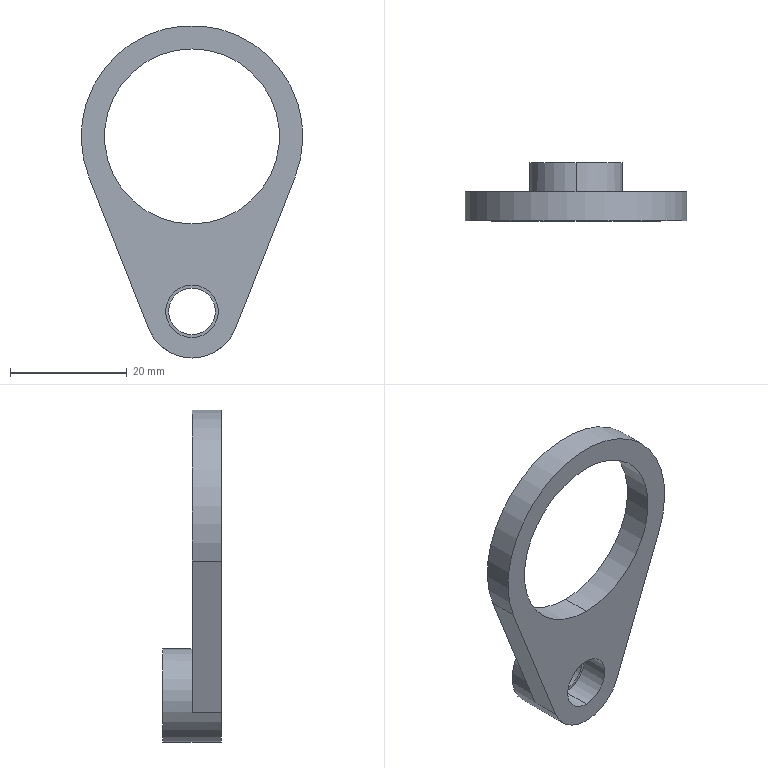Part | SolidWorks | features ICE 3, Extrusion 1 | 1 solid | 15 faces | box 38 x 10 x 57 mm | volume 4565 mm3 | cylinder 9 | plane 6 | commonest cylinder face diameters 8 x2 9 x2 16 x2 30 x2 38 x1
STEP:
#1=CARTESIAN_POINT('',(0.,5.,4.5));
#2=VERTEX_POINT('',#1);
#3=CARTESIAN_POINT('',(0.,5.,-4.5));
#4=VERTEX_POINT('',#3);
#5=CARTESIAN_POINT('',(0.,5.,0.));
#6=DIRECTION('',(0.,-1.,0.));
#7=DIRECTION('',(0.,0.,-1.));
#8=AXIS2_PLACEMENT_3D('',#5,#6,#7);
#9=CIRCLE('',#8,4.5);
#10=EDGE_CURVE('',#2,#4,#9,.T.);
#11=ORIENTED_EDGE('',*,*,#10,.F.);
#12=CARTESIAN_POINT('',(0.,0.,4.5));
#13=VERTEX_POINT('',#12);
#14=CARTESIAN_POINT('',(0.,5.,4.5));
#15=DIRECTION('',(0.,-1.,0.));
#16=VECTOR('',#15,1000.);
#17=LINE('',#14,#16);
#18=EDGE_CURVE('',#2,#13,#17,.T.);
#19=ORIENTED_EDGE('',*,*,#18,.T.);
#20=CARTESIAN_POINT('',(0.,0.,-4.5));
#21=VERTEX_POINT('',#20);
#22=CARTESIAN_POINT('',(0.,0.,0.));
#23=DIRECTION('',(0.,-1.,0.));
#24=DIRECTION('',(0.,0.,-1.));
#25=AXIS2_PLACEMENT_3D('',#22,#23,#24);
#26=CIRCLE('',#25,4.5);
#27=EDGE_CURVE('',#13,#21,#26,.T.);
#28=ORIENTED_EDGE('',*,*,#27,.T.);
#29=CARTESIAN_POINT('',(0.,5.,-4.5));
#30=DIRECTION('',(0.,-1.,0.));
#31=VECTOR('',#30,1000.);
#32=LINE('',#29,#31);
#33=EDGE_CURVE('',#4,#21,#32,.T.);
#34=ORIENTED_EDGE('',*,*,#33,.F.);
#35=EDGE_LOOP('',(#11,#19,#28,#34));
#36=FACE_OUTER_BOUND('',#35,.T.);
#37=CARTESIAN_POINT('',(0.,5.,0.));
#38=DIRECTION('',(0.,-1.,0.));
#39=DIRECTION('',(0.,0.,-1.));
#40=AXIS2_PLACEMENT_3D('',#37,#38,#39);
#41=CYLINDRICAL_SURFACE('',#40,4.5);
#42=ADVANCED_FACE('',(#36),#41,.F.);
#43=CARTESIAN_POINT('',(0.,0.,15.));
#44=VERTEX_POINT('',#43);
#45=CARTESIAN_POINT('',(0.,0.,45.));
#46=VERTEX_POINT('',#45);
#47=CARTESIAN_POINT('',(0.,0.,30.));
#48=DIRECTION('',(0.,1.,0.));
#49=DIRECTION('',(0.,0.,1.));
#50=AXIS2_PLACEMENT_3D('',#47,#48,#49);
#51=CIRCLE('',#50,15.);
#52=EDGE_CURVE('',#44,#46,#51,.T.);
#53=ORIENTED_EDGE('',*,*,#52,.F.);
#54=CARTESIAN_POINT('',(0.,5.,15.));
#55=VERTEX_POINT('',#54);
#56=CARTESIAN_POINT('',(0.,-29.,15.));
#57=DIRECTION('',(0.,1.,0.));
#58=VECTOR('',#57,1000.);
#59=LINE('',#56,#58);
#60=EDGE_CURVE('',#44,#55,#59,.T.);
#61=ORIENTED_EDGE('',*,*,#60,.T.);
#62=CARTESIAN_POINT('',(0.,5.,45.));
#63=VERTEX_POINT('',#62);
#64=CARTESIAN_POINT('',(0.,5.,30.));
#65=DIRECTION('',(0.,1.,0.));
#66=DIRECTION('',(0.,0.,1.));
#67=AXIS2_PLACEMENT_3D('',#64,#65,#66);
#68=CIRCLE('',#67,15.);
#69=EDGE_CURVE('',#55,#63,#68,.T.);
#70=ORIENTED_EDGE('',*,*,#69,.T.);
#71=CARTESIAN_POINT('',(0.,-29.,45.));
#72=DIRECTION('',(0.,1.,0.));
#73=VECTOR('',#72,1000.);
#74=LINE('',#71,#73);
#75=EDGE_CURVE('',#46,#63,#74,.T.);
#76=ORIENTED_EDGE('',*,*,#75,.F.);
#77=EDGE_LOOP('',(#53,#61,#70,#76));
#78=FACE_OUTER_BOUND('',#77,.T.);
#79=CARTESIAN_POINT('',(0.,-29.,30.));
#80=DIRECTION('',(0.,1.,0.));
#81=DIRECTION('',(0.,0.,1.));
#82=AXIS2_PLACEMENT_3D('',#79,#80,#81);
#83=CYLINDRICAL_SURFACE('',#82,15.);
#84=ADVANCED_FACE('',(#78),#83,.F.);
#85=CARTESIAN_POINT('',(0.,10.,8.));
#86=VERTEX_POINT('',#85);
#87=CARTESIAN_POINT('',(0.,10.,-8.));
#88=VERTEX_POINT('',#87);
#89=CARTESIAN_POINT('',(0.,10.,0.));
#90=DIRECTION('',(0.,1.,0.));
#91=DIRECTION('',(0.,0.,1.));
#92=AXIS2_PLACEMENT_3D('',#89,#90,#91);
#93=CIRCLE('',#92,8.);
#94=EDGE_CURVE('',#86,#88,#93,.T.);
#95=ORIENTED_EDGE('',*,*,#94,.F.);
#96=CARTESIAN_POINT('',(0.,5.,8.));
#97=VERTEX_POINT('',#96);
#98=CARTESIAN_POINT('',(0.,5.,8.));
#99=DIRECTION('',(0.,-1.,0.));
#100=VECTOR('',#99,1000.);
#101=LINE('',#98,#100);
#102=EDGE_CURVE('',#86,#97,#101,.T.);
#103=ORIENTED_EDGE('',*,*,#102,.T.);
#104=CARTESIAN_POINT('',(7.443,5.,-2.933));
#105=VERTEX_POINT('',#104);
#106=CARTESIAN_POINT('',(0.,5.,0.));
#107=DIRECTION('',(0.,1.,0.));
#108=DIRECTION('',(0.,0.,1.));
#109=AXIS2_PLACEMENT_3D('',#106,#107,#108);
#110=CIRCLE('',#109,8.);
#111=EDGE_CURVE('',#97,#105,#110,.T.);
#112=ORIENTED_EDGE('',*,*,#111,.T.);
#113=CARTESIAN_POINT('',(7.443,0.,-2.933));
#114=VERTEX_POINT('',#113);
#115=CARTESIAN_POINT('',(7.443,5.,-2.933));
#116=DIRECTION('',(0.,-1.,0.));
#117=VECTOR('',#116,1000.);
#118=LINE('',#115,#117);
#119=EDGE_CURVE('',#105,#114,#118,.T.);
#120=ORIENTED_EDGE('',*,*,#119,.T.);
#121=CARTESIAN_POINT('',(0.,0.,-8.));
#122=VERTEX_POINT('',#121);
#123=CARTESIAN_POINT('',(0.,0.,0.));
#124=DIRECTION('',(0.,1.,0.));
#125=DIRECTION('',(0.,0.,1.));
#126=AXIS2_PLACEMENT_3D('',#123,#124,#125);
#127=CIRCLE('',#126,8.);
#128=EDGE_CURVE('',#114,#122,#127,.T.);
#129=ORIENTED_EDGE('',*,*,#128,.T.);
#130=CARTESIAN_POINT('',(0.,5.,-8.));
#131=DIRECTION('',(0.,-1.,0.));
#132=VECTOR('',#131,1000.);
#133=LINE('',#130,#132);
#134=EDGE_CURVE('',#88,#122,#133,.T.);
#135=ORIENTED_EDGE('',*,*,#134,.F.);
#136=EDGE_LOOP('',(#95,#103,#112,#120,#129,#135));
#137=FACE_OUTER_BOUND('',#136,.T.);
#138=CARTESIAN_POINT('',(0.,5.,0.));
#139=DIRECTION('',(0.,-1.,0.));
#140=DIRECTION('',(0.,0.,-1.));
#141=AXIS2_PLACEMENT_3D('',#138,#139,#140);
#142=CYLINDRICAL_SURFACE('',#141,8.);
#143=ADVANCED_FACE('',(#137),#142,.T.);
#144=CARTESIAN_POINT('',(0.,5.,-4.));
#145=VERTEX_POINT('',#144);
#146=CARTESIAN_POINT('',(0.,5.,4.));
#147=VERTEX_POINT('',#146);
#148=CARTESIAN_POINT('',(0.,5.,0.));
#149=DIRECTION('',(0.,1.,0.));
#150=DIRECTION('',(0.,0.,-1.));
#151=AXIS2_PLACEMENT_3D('',#148,#149,#150);
#152=CIRCLE('',#151,4.);
#153=EDGE_CURVE('',#145,#147,#152,.T.);
#154=ORIENTED_EDGE('',*,*,#153,.F.);
#155=CARTESIAN_POINT('',(0.,10.,-4.));
#156=VERTEX_POINT('',#155);
#157=CARTESIAN_POINT('',(0.,-29.,-4.));
#158=DIRECTION('',(0.,1.,0.));
#159=VECTOR('',#158,1000.);
#160=LINE('',#157,#159);
#161=EDGE_CURVE('',#145,#156,#160,.T.);
#162=ORIENTED_EDGE('',*,*,#161,.T.);
#163=CARTESIAN_POINT('',(0.,10.,4.));
#164=VERTEX_POINT('',#163);
#165=CARTESIAN_POINT('',(0.,10.,0.));
#166=DIRECTION('',(0.,1.,0.));
#167=DIRECTION('',(0.,0.,1.));
#168=AXIS2_PLACEMENT_3D('',#165,#166,#167);
#169=CIRCLE('',#168,4.);
#170=EDGE_CURVE('',#156,#164,#169,.T.);
#171=ORIENTED_EDGE('',*,*,#170,.T.);
#172=CARTESIAN_POINT('',(0.,-29.,4.));
#173=DIRECTION('',(0.,1.,0.));
#174=VECTOR('',#173,1000.);
#175=LINE('',#172,#174);
#176=EDGE_CURVE('',#147,#164,#175,.T.);
#177=ORIENTED_EDGE('',*,*,#176,.F.);
#178=EDGE_LOOP('',(#154,#162,#171,#177));
#179=FACE_OUTER_BOUND('',#178,.T.);
#180=CARTESIAN_POINT('',(0.,-29.,0.));
#181=DIRECTION('',(0.,1.,0.));
#182=DIRECTION('',(0.,0.,1.));
#183=AXIS2_PLACEMENT_3D('',#180,#181,#182);
#184=CYLINDRICAL_SURFACE('',#183,4.);
#185=ADVANCED_FACE('',(#179),#184,.F.);
#186=ORIENTED_EDGE('',*,*,#161,.F.);
#187=CARTESIAN_POINT('',(0.,5.,0.));
#188=DIRECTION('',(0.,1.,0.));
#189=DIRECTION('',(0.,0.,-1.));
#190=AXIS2_PLACEMENT_3D('',#187,#188,#189);
#191=CIRCLE('',#190,4.);
#192=EDGE_CURVE('',#147,#145,#191,.T.);
#193=ORIENTED_EDGE('',*,*,#192,.F.);
#194=ORIENTED_EDGE('',*,*,#176,.T.);
#195=CARTESIAN_POINT('',(0.,10.,0.));
#196=DIRECTION('',(0.,1.,0.));
#197=DIRECTION('',(0.,0.,1.));
#198=AXIS2_PLACEMENT_3D('',#195,#196,#197);
#199=CIRCLE('',#198,4.);
#200=EDGE_CURVE('',#164,#156,#199,.T.);
#201=ORIENTED_EDGE('',*,*,#200,.T.);
#202=EDGE_LOOP('',(#186,#193,#194,#201));
#203=FACE_OUTER_BOUND('',#202,.T.);
#204=CARTESIAN_POINT('',(0.,-29.,0.));
#205=DIRECTION('',(0.,1.,0.));
#206=DIRECTION('',(0.,0.,1.));
#207=AXIS2_PLACEMENT_3D('',#204,#205,#206);
#208=CYLINDRICAL_SURFACE('',#207,4.);
#209=ADVANCED_FACE('',(#203),#208,.F.);
#210=ORIENTED_EDGE('',*,*,#102,.F.);
#211=CARTESIAN_POINT('',(0.,10.,0.));
#212=DIRECTION('',(0.,1.,0.));
#213=DIRECTION('',(0.,0.,1.));
#214=AXIS2_PLACEMENT_3D('',#211,#212,#213);
#215=CIRCLE('',#214,8.);
#216=EDGE_CURVE('',#88,#86,#215,.T.);
#217=ORIENTED_EDGE('',*,*,#216,.F.);
#218=ORIENTED_EDGE('',*,*,#134,.T.);
#219=CARTESIAN_POINT('',(-7.443,0.,-2.933));
#220=VERTEX_POINT('',#219);
#221=CARTESIAN_POINT('',(0.,0.,0.));
#222=DIRECTION('',(0.,1.,0.));
#223=DIRECTION('',(0.,0.,1.));
#224=AXIS2_PLACEMENT_3D('',#221,#222,#223);
#225=CIRCLE('',#224,8.);
#226=EDGE_CURVE('',#122,#220,#225,.T.);
#227=ORIENTED_EDGE('',*,*,#226,.T.);
#228=CARTESIAN_POINT('',(-7.443,5.,-2.933));
#229=VERTEX_POINT('',#228);
#230=CARTESIAN_POINT('',(-7.443,5.,-2.933));
#231=DIRECTION('',(0.,-1.,0.));
#232=VECTOR('',#231,1000.);
#233=LINE('',#230,#232);
#234=EDGE_CURVE('',#229,#220,#233,.T.);
#235=ORIENTED_EDGE('',*,*,#234,.F.);
#236=CARTESIAN_POINT('',(0.,5.,0.));
#237=DIRECTION('',(0.,1.,0.));
#238=DIRECTION('',(0.,0.,1.));
#239=AXIS2_PLACEMENT_3D('',#236,#237,#238);
#240=CIRCLE('',#239,8.);
#241=EDGE_CURVE('',#229,#97,#240,.T.);
#242=ORIENTED_EDGE('',*,*,#241,.T.);
#243=EDGE_LOOP('',(#210,#217,#218,#227,#235,#242));
#244=FACE_OUTER_BOUND('',#243,.T.);
#245=CARTESIAN_POINT('',(0.,5.,0.));
#246=DIRECTION('',(0.,-1.,0.));
#247=DIRECTION('',(0.,0.,-1.));
#248=AXIS2_PLACEMENT_3D('',#245,#246,#247);
#249=CYLINDRICAL_SURFACE('',#248,8.);
#250=ADVANCED_FACE('',(#244),#249,.T.);
#251=CARTESIAN_POINT('',(-17.677,0.,23.033));
#252=VERTEX_POINT('',#251);
#253=CARTESIAN_POINT('',(-7.443,0.,-2.933));
#254=DIRECTION('',(-0.3667,0.,0.9304));
#255=VECTOR('',#254,1000.);
#256=LINE('',#253,#255);
#257=EDGE_CURVE('',#220,#252,#256,.T.);
#258=ORIENTED_EDGE('',*,*,#257,.T.);
#259=CARTESIAN_POINT('',(-17.677,5.,23.033));
#260=VERTEX_POINT('',#259);
#261=CARTESIAN_POINT('',(-17.677,5.,23.033));
#262=DIRECTION('',(0.,-1.,0.));
#263=VECTOR('',#262,1000.);
#264=LINE('',#261,#263);
#265=EDGE_CURVE('',#260,#252,#264,.T.);
#266=ORIENTED_EDGE('',*,*,#265,.F.);
#267=CARTESIAN_POINT('',(-7.443,5.,-2.933));
#268=DIRECTION('',(-0.3667,0.,0.9304));
#269=VECTOR('',#268,1000.);
#270=LINE('',#267,#269);
#271=EDGE_CURVE('',#229,#260,#270,.T.);
#272=ORIENTED_EDGE('',*,*,#271,.F.);
#273=ORIENTED_EDGE('',*,*,#234,.T.);
#274=EDGE_LOOP('',(#258,#266,#272,#273));
#275=FACE_OUTER_BOUND('',#274,.T.);
#276=CARTESIAN_POINT('',(-7.443,5.,-2.933));
#277=DIRECTION('',(0.9304,0.,0.3667));
#278=DIRECTION('',(0.3667,0.,-0.9304));
#279=AXIS2_PLACEMENT_3D('',#276,#277,#278);
#280=PLANE('',#279);
#281=ADVANCED_FACE('',(#275),#280,.F.);
#282=CARTESIAN_POINT('',(17.677,0.,23.033));
#283=VERTEX_POINT('',#282);
#284=CARTESIAN_POINT('',(0.,0.,30.));
#285=DIRECTION('',(0.,1.,0.));
#286=DIRECTION('',(0.,0.,1.));
#287=AXIS2_PLACEMENT_3D('',#284,#285,#286);
#288=CIRCLE('',#287,19.);
#289=EDGE_CURVE('',#252,#283,#288,.T.);
#290=ORIENTED_EDGE('',*,*,#289,.T.);
#291=CARTESIAN_POINT('',(17.677,5.,23.033));
#292=VERTEX_POINT('',#291);
#293=CARTESIAN_POINT('',(17.677,5.,23.033));
#294=DIRECTION('',(0.,-1.,0.));
#295=VECTOR('',#294,1000.);
#296=LINE('',#293,#295);
#297=EDGE_CURVE('',#292,#283,#296,.T.);
#298=ORIENTED_EDGE('',*,*,#297,.F.);
#299=CARTESIAN_POINT('',(0.,5.,30.));
#300=DIRECTION('',(0.,1.,0.));
#301=DIRECTION('',(0.,0.,1.));
#302=AXIS2_PLACEMENT_3D('',#299,#300,#301);
#303=CIRCLE('',#302,19.);
#304=EDGE_CURVE('',#260,#292,#303,.T.);
#305=ORIENTED_EDGE('',*,*,#304,.F.);
#306=ORIENTED_EDGE('',*,*,#265,.T.);
#307=EDGE_LOOP('',(#290,#298,#305,#306));
#308=FACE_OUTER_BOUND('',#307,.T.);
#309=CARTESIAN_POINT('',(0.,5.,30.));
#310=DIRECTION('',(0.,-1.,0.));
#311=DIRECTION('',(0.,0.,-1.));
#312=AXIS2_PLACEMENT_3D('',#309,#310,#311);
#313=CYLINDRICAL_SURFACE('',#312,19.);
#314=ADVANCED_FACE('',(#308),#313,.T.);
#315=CARTESIAN_POINT('',(7.443,0.,-2.933));
#316=DIRECTION('',(-0.3667,0.,-0.9304));
#317=VECTOR('',#316,1000.);
#318=LINE('',#315,#317);
#319=EDGE_CURVE('',#283,#114,#318,.T.);
#320=ORIENTED_EDGE('',*,*,#319,.T.);
#321=ORIENTED_EDGE('',*,*,#119,.F.);
#322=CARTESIAN_POINT('',(7.443,5.,-2.933));
#323=DIRECTION('',(-0.3667,0.,-0.9304));
#324=VECTOR('',#323,1000.);
#325=LINE('',#322,#324);
#326=EDGE_CURVE('',#292,#105,#325,.T.);
#327=ORIENTED_EDGE('',*,*,#326,.F.);
#328=ORIENTED_EDGE('',*,*,#297,.T.);
#329=EDGE_LOOP('',(#320,#321,#327,#328));
#330=FACE_OUTER_BOUND('',#329,.T.);
#331=CARTESIAN_POINT('',(7.443,5.,-2.933));
#332=DIRECTION('',(-0.9304,0.,0.3667));
#333=DIRECTION('',(0.3667,0.,0.9304));
#334=AXIS2_PLACEMENT_3D('',#331,#332,#333);
#335=PLANE('',#334);
#336=ADVANCED_FACE('',(#330),#335,.F.);
#337=CARTESIAN_POINT('',(0.,5.,30.));
#338=DIRECTION('',(0.,1.,0.));
#339=DIRECTION('',(0.,0.,1.));
#340=AXIS2_PLACEMENT_3D('',#337,#338,#339);
#341=CIRCLE('',#340,15.);
#342=EDGE_CURVE('',#63,#55,#341,.T.);
#343=ORIENTED_EDGE('',*,*,#342,.F.);
#344=ORIENTED_EDGE('',*,*,#69,.F.);
#345=EDGE_LOOP('',(#343,#344));
#346=FACE_BOUND('',#345,.T.);
#347=ORIENTED_EDGE('',*,*,#241,.F.);
#348=ORIENTED_EDGE('',*,*,#271,.T.);
#349=ORIENTED_EDGE('',*,*,#304,.T.);
#350=ORIENTED_EDGE('',*,*,#326,.T.);
#351=ORIENTED_EDGE('',*,*,#111,.F.);
#352=EDGE_LOOP('',(#347,#348,#349,#350,#351));
#353=FACE_OUTER_BOUND('',#352,.T.);
#354=CARTESIAN_POINT('',(0.,5.,0.));
#355=DIRECTION('',(0.,1.,0.));
#356=DIRECTION('',(0.,0.,1.));
#357=AXIS2_PLACEMENT_3D('',#354,#355,#356);
#358=PLANE('',#357);
#359=ADVANCED_FACE('',(#346,#353),#358,.T.);
#360=CARTESIAN_POINT('',(0.,0.,0.));
#361=DIRECTION('',(0.,-1.,0.));
#362=DIRECTION('',(0.,0.,-1.));
#363=AXIS2_PLACEMENT_3D('',#360,#361,#362);
#364=CIRCLE('',#363,4.5);
#365=EDGE_CURVE('',#21,#13,#364,.T.);
#366=ORIENTED_EDGE('',*,*,#365,.F.);
#367=ORIENTED_EDGE('',*,*,#27,.F.);
#368=EDGE_LOOP('',(#366,#367));
#369=FACE_BOUND('',#368,.T.);
#370=CARTESIAN_POINT('',(0.,0.,30.));
#371=DIRECTION('',(0.,1.,0.));
#372=DIRECTION('',(0.,0.,1.));
#373=AXIS2_PLACEMENT_3D('',#370,#371,#372);
#374=CIRCLE('',#373,15.);
#375=EDGE_CURVE('',#46,#44,#374,.T.);
#376=ORIENTED_EDGE('',*,*,#375,.T.);
#377=ORIENTED_EDGE('',*,*,#52,.T.);
#378=EDGE_LOOP('',(#376,#377));
#379=FACE_BOUND('',#378,.T.);
#380=ORIENTED_EDGE('',*,*,#128,.F.);
#381=ORIENTED_EDGE('',*,*,#319,.F.);
#382=ORIENTED_EDGE('',*,*,#289,.F.);
#383=ORIENTED_EDGE('',*,*,#257,.F.);
#384=ORIENTED_EDGE('',*,*,#226,.F.);
#385=EDGE_LOOP('',(#380,#381,#382,#383,#384));
#386=FACE_OUTER_BOUND('',#385,.T.);
#387=CARTESIAN_POINT('',(0.,0.,0.));
#388=DIRECTION('',(0.,1.,0.));
#389=DIRECTION('',(0.,0.,1.));
#390=AXIS2_PLACEMENT_3D('',#387,#388,#389);
#391=PLANE('',#390);
#392=ADVANCED_FACE('',(#369,#379,#386),#391,.F.);
#393=ORIENTED_EDGE('',*,*,#200,.F.);
#394=ORIENTED_EDGE('',*,*,#170,.F.);
#395=EDGE_LOOP('',(#393,#394));
#396=FACE_BOUND('',#395,.T.);
#397=ORIENTED_EDGE('',*,*,#216,.T.);
#398=ORIENTED_EDGE('',*,*,#94,.T.);
#399=EDGE_LOOP('',(#397,#398));
#400=FACE_OUTER_BOUND('',#399,.T.);
#401=CARTESIAN_POINT('',(0.,10.,0.));
#402=DIRECTION('',(0.,1.,0.));
#403=DIRECTION('',(0.,0.,1.));
#404=AXIS2_PLACEMENT_3D('',#401,#402,#403);
#405=PLANE('',#404);
#406=ADVANCED_FACE('',(#396,#400),#405,.T.);
#407=ORIENTED_EDGE('',*,*,#60,.F.);
#408=ORIENTED_EDGE('',*,*,#375,.F.);
#409=ORIENTED_EDGE('',*,*,#75,.T.);
#410=ORIENTED_EDGE('',*,*,#342,.T.);
#411=EDGE_LOOP('',(#407,#408,#409,#410));
#412=FACE_OUTER_BOUND('',#411,.T.);
#413=CARTESIAN_POINT('',(0.,-29.,30.));
#414=DIRECTION('',(0.,1.,0.));
#415=DIRECTION('',(0.,0.,1.));
#416=AXIS2_PLACEMENT_3D('',#413,#414,#415);
#417=CYLINDRICAL_SURFACE('',#416,15.);
#418=ADVANCED_FACE('',(#412),#417,.F.);
#419=CARTESIAN_POINT('',(0.,5.,0.));
#420=DIRECTION('',(0.,-1.,0.));
#421=DIRECTION('',(0.,0.,-1.));
#422=AXIS2_PLACEMENT_3D('',#419,#420,#421);
#423=CIRCLE('',#422,4.5);
#424=EDGE_CURVE('',#4,#2,#423,.T.);
#425=ORIENTED_EDGE('',*,*,#424,.T.);
#426=ORIENTED_EDGE('',*,*,#10,.T.);
#427=EDGE_LOOP('',(#425,#426));
#428=FACE_OUTER_BOUND('',#427,.T.);
#429=ORIENTED_EDGE('',*,*,#192,.T.);
#430=ORIENTED_EDGE('',*,*,#153,.T.);
#431=EDGE_LOOP('',(#429,#430));
#432=FACE_BOUND('',#431,.T.);
#433=CARTESIAN_POINT('',(0.,5.,0.));
#434=DIRECTION('',(0.,-1.,0.));
#435=DIRECTION('',(0.,0.,-1.));
#436=AXIS2_PLACEMENT_3D('',#433,#434,#435);
#437=PLANE('',#436);
#438=ADVANCED_FACE('',(#428,#432),#437,.T.);
#439=ORIENTED_EDGE('',*,*,#18,.F.);
#440=ORIENTED_EDGE('',*,*,#424,.F.);
#441=ORIENTED_EDGE('',*,*,#33,.T.);
#442=ORIENTED_EDGE('',*,*,#365,.T.);
#443=EDGE_LOOP('',(#439,#440,#441,#442));
#444=FACE_OUTER_BOUND('',#443,.T.);
#445=CARTESIAN_POINT('',(0.,5.,0.));
#446=DIRECTION('',(0.,-1.,0.));
#447=DIRECTION('',(0.,0.,-1.));
#448=AXIS2_PLACEMENT_3D('',#445,#446,#447);
#449=CYLINDRICAL_SURFACE('',#448,4.5);
#450=ADVANCED_FACE('',(#444),#449,.F.);
#451=CLOSED_SHELL('',(#42,#84,#143,#185,#209,#250,#281,#314,#336,#359,#392,#406,#418,#438,#450));
#452=MANIFOLD_SOLID_BREP('',#451);
#453=CARTESIAN_POINT('',(0.,0.,0.));
#454=DIRECTION('',(0.,0.,1.));
#455=DIRECTION('',(1.,0.,0.));
#456=AXIS2_PLACEMENT_3D('',#453,#454,#455);
#457=(LENGTH_UNIT()NAMED_UNIT(*)SI_UNIT(.MILLI.,.METRE.));
#458=UNCERTAINTY_MEASURE_WITH_UNIT(LENGTH_MEASURE(0.00001),#457,'','');
#459=(NAMED_UNIT(*)PLANE_ANGLE_UNIT()SI_UNIT($,.RADIAN.));
#460=(NAMED_UNIT(*)SI_UNIT($,.STERADIAN.)SOLID_ANGLE_UNIT());
#461=(GEOMETRIC_REPRESENTATION_CONTEXT(3)GLOBAL_UNCERTAINTY_ASSIGNED_CONTEXT((#458))GLOBAL_UNIT_ASSIGNED_CONTEXT((#457,#459,#460))REPRESENTATION_CONTEXT('',''));
#462=ADVANCED_BREP_SHAPE_REPRESENTATION('',(#452,#456),#461);